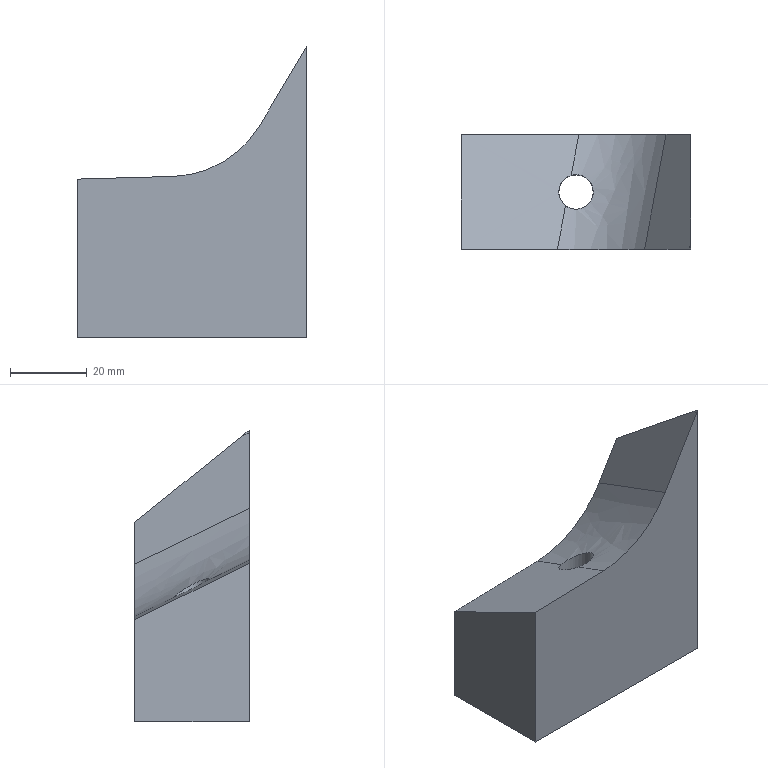Part | NX | features solid 2 | 1 solid | 10 faces | box 60.003 x 30 x 76.186 mm | volume 68995 mm3 | plane 5 | spline 4 | cylinder 1 | commonest cylinder face diameters 9 x1
STEP:
#1=CARTESIAN_POINT('',(-584.5,125.,-55.));
#2=VERTEX_POINT('',#1);
#3=CARTESIAN_POINT('',(-580.,125.,-55.));
#4=DIRECTION('',(0.,0.,-1.));
#5=DIRECTION('',(-1.,0.,0.));
#6=AXIS2_PLACEMENT_3D('',#3,#4,#5);
#7=CIRCLE('',#6,4.5);
#8=EDGE_CURVE('',#2,#2,#7,.T.);
#9=ORIENTED_EDGE('',*,*,#8,.F.);
#10=EDGE_LOOP('',(#9));
#11=FACE_BOUND('',#10,.T.);
#12=CARTESIAN_POINT('',(-610.,140.,-55.));
#13=VERTEX_POINT('',#12);
#14=CARTESIAN_POINT('',(-550.,140.,-55.));
#15=VERTEX_POINT('',#14);
#16=CARTESIAN_POINT('',(-615.,140.,-55.));
#17=DIRECTION('',(1.,0.,0.));
#18=VECTOR('',#17,1000.);
#19=LINE('',#16,#18);
#20=EDGE_CURVE('',#13,#15,#19,.T.);
#21=ORIENTED_EDGE('',*,*,#20,.T.);
#22=CARTESIAN_POINT('',(-550.,110.,-55.));
#23=VERTEX_POINT('',#22);
#24=CARTESIAN_POINT('',(-550.,140.,-55.));
#25=DIRECTION('',(0.,-1.,0.));
#26=VECTOR('',#25,1000.);
#27=LINE('',#24,#26);
#28=EDGE_CURVE('',#15,#23,#27,.T.);
#29=ORIENTED_EDGE('',*,*,#28,.T.);
#30=CARTESIAN_POINT('',(-610.,110.,-55.));
#31=VERTEX_POINT('',#30);
#32=CARTESIAN_POINT('',(-540.,110.,-55.));
#33=DIRECTION('',(-1.,0.,0.));
#34=VECTOR('',#33,1000.);
#35=LINE('',#32,#34);
#36=EDGE_CURVE('',#23,#31,#35,.T.);
#37=ORIENTED_EDGE('',*,*,#36,.T.);
#38=CARTESIAN_POINT('',(-610.,110.,-55.));
#39=DIRECTION('',(0.,1.,0.));
#40=VECTOR('',#39,1000.);
#41=LINE('',#38,#40);
#42=EDGE_CURVE('',#31,#13,#41,.T.);
#43=ORIENTED_EDGE('',*,*,#42,.T.);
#44=EDGE_LOOP('',(#21,#29,#37,#43));
#45=FACE_BOUND('',#44,.T.);
#46=CARTESIAN_POINT('',(-540.,140.,-55.));
#47=DIRECTION('',(0.,0.,-1.));
#48=DIRECTION('',(-1.,0.,0.));
#49=AXIS2_PLACEMENT_3D('',#46,#47,#48);
#50=PLANE('',#49);
#51=ADVANCED_FACE('',(#11,#45),#50,.T.);
#52=CARTESIAN_POINT('',(-610.,110.,-13.535));
#53=VERTEX_POINT('',#52);
#54=CARTESIAN_POINT('',(-610.,110.,-50.));
#55=DIRECTION('',(0.,0.,1.));
#56=VECTOR('',#55,1000.);
#57=LINE('',#54,#56);
#58=EDGE_CURVE('',#31,#53,#57,.T.);
#59=ORIENTED_EDGE('',*,*,#58,.T.);
#60=CARTESIAN_POINT('',(-610.,140.,-28.38));
#61=VERTEX_POINT('',#60);
#62=CARTESIAN_POINT('',(-610.,124.496,-20.708));
#63=DIRECTION('',(0.,-0.8963,0.4435));
#64=VECTOR('',#63,1000.);
#65=LINE('',#62,#64);
#66=EDGE_CURVE('',#53,#61,#65,.F.);
#67=ORIENTED_EDGE('',*,*,#66,.T.);
#68=CARTESIAN_POINT('',(-610.,140.,-50.));
#69=DIRECTION('',(0.,0.,1.));
#70=VECTOR('',#69,1000.);
#71=LINE('',#68,#70);
#72=EDGE_CURVE('',#13,#61,#71,.T.);
#73=ORIENTED_EDGE('',*,*,#72,.F.);
#74=ORIENTED_EDGE('',*,*,#42,.F.);
#75=EDGE_LOOP('',(#59,#67,#73,#74));
#76=FACE_BOUND('',#75,.T.);
#77=CARTESIAN_POINT('',(-610.,110.,-50.));
#78=DIRECTION('',(1.,0.,0.));
#79=DIRECTION('',(0.,0.,-1.));
#80=AXIS2_PLACEMENT_3D('',#77,#78,#79);
#81=PLANE('',#80);
#82=ADVANCED_FACE('',(#76),#81,.F.);
#83=CARTESIAN_POINT('',(-562.096,110.,0.8233));
#84=VERTEX_POINT('',#83);
#85=CARTESIAN_POINT('',(-584.853,110.,-12.829));
#86=VERTEX_POINT('',#85);
#87=CARTESIAN_POINT('',(-562.096,110.,0.8233));
#88=CARTESIAN_POINT('',(-564.471,110.,-3.178));
#89=CARTESIAN_POINT('',(-569.402,110.,-8.281));
#90=CARTESIAN_POINT('',(-577.942,110.,-12.047));
#91=CARTESIAN_POINT('',(-582.526,110.,-12.763));
#92=CARTESIAN_POINT('',(-584.853,110.,-12.829));
#93=B_SPLINE_CURVE_WITH_KNOTS('',3,(#87,#88,#89,#90,#91,#92),.UNSPECIFIED.,.F.,.F.,(4,1,1,4),(0.,0.01386,0.02078,0.02771),.UNSPECIFIED.);
#94=EDGE_CURVE('',#84,#86,#93,.T.);
#95=ORIENTED_EDGE('',*,*,#94,.T.);
#96=CARTESIAN_POINT('',(-541.078,110.,-11.6));
#97=DIRECTION('',(0.9996,0.,0.02806));
#98=VECTOR('',#97,1000.);
#99=LINE('',#96,#98);
#100=EDGE_CURVE('',#86,#53,#99,.F.);
#101=ORIENTED_EDGE('',*,*,#100,.T.);
#102=ORIENTED_EDGE('',*,*,#58,.F.);
#103=ORIENTED_EDGE('',*,*,#36,.F.);
#104=CARTESIAN_POINT('',(-550.,110.,21.186));
#105=VERTEX_POINT('',#104);
#106=CARTESIAN_POINT('',(-550.,110.,-50.));
#107=DIRECTION('',(0.,0.,1.));
#108=VECTOR('',#107,1000.);
#109=LINE('',#106,#108);
#110=EDGE_CURVE('',#23,#105,#109,.T.);
#111=ORIENTED_EDGE('',*,*,#110,.T.);
#112=CARTESIAN_POINT('',(-550.378,110.,20.569));
#113=VERTEX_POINT('',#112);
#114=CARTESIAN_POINT('',(-550.,110.,21.186));
#115=CARTESIAN_POINT('',(-550.129,110.,20.981));
#116=CARTESIAN_POINT('',(-550.256,110.,20.773));
#117=CARTESIAN_POINT('',(-550.38,110.,20.564));
#118=B_SPLINE_CURVE_WITH_KNOTS('',3,(#114,#115,#116,#117),.UNSPECIFIED.,.F.,.F.,(4,4),(0.,0.0007289),.UNSPECIFIED.);
#119=EDGE_CURVE('',#105,#113,#118,.T.);
#120=ORIENTED_EDGE('',*,*,#119,.T.);
#121=CARTESIAN_POINT('',(-578.647,110.,-27.064));
#122=DIRECTION('',(0.5104,0.,0.86));
#123=VECTOR('',#122,1000.);
#124=LINE('',#121,#123);
#125=EDGE_CURVE('',#113,#84,#124,.F.);
#126=ORIENTED_EDGE('',*,*,#125,.T.);
#127=EDGE_LOOP('',(#95,#101,#102,#103,#111,#120,#126));
#128=FACE_BOUND('',#127,.T.);
#129=CARTESIAN_POINT('',(-540.,110.,-50.));
#130=DIRECTION('',(0.,1.,0.));
#131=DIRECTION('',(0.,0.,1.));
#132=AXIS2_PLACEMENT_3D('',#129,#130,#131);
#133=PLANE('',#132);
#134=ADVANCED_FACE('',(#128),#133,.F.);
#135=CARTESIAN_POINT('',(-550.,140.,-2.908));
#136=VERTEX_POINT('',#135);
#137=CARTESIAN_POINT('',(-550.,140.,-50.));
#138=DIRECTION('',(0.,0.,1.));
#139=VECTOR('',#138,1000.);
#140=LINE('',#137,#139);
#141=EDGE_CURVE('',#15,#136,#140,.T.);
#142=ORIENTED_EDGE('',*,*,#141,.T.);
#143=CARTESIAN_POINT('',(-550.,111.813,19.748));
#144=VERTEX_POINT('',#143);
#145=CARTESIAN_POINT('',(-550.,162.995,-21.39));
#146=DIRECTION('',(0.,0.7794,-0.6265));
#147=VECTOR('',#146,1000.);
#148=LINE('',#145,#147);
#149=EDGE_CURVE('',#136,#144,#148,.F.);
#150=ORIENTED_EDGE('',*,*,#149,.T.);
#151=CARTESIAN_POINT('',(-550.,111.819,19.743));
#152=CARTESIAN_POINT('',(-550.,111.216,20.228));
#153=CARTESIAN_POINT('',(-550.,110.609,20.709));
#154=CARTESIAN_POINT('',(-550.,110.,21.186));
#155=B_SPLINE_CURVE_WITH_KNOTS('',3,(#151,#152,#153,#154),.UNSPECIFIED.,.F.,.F.,(4,4),(0.,0.002322),.UNSPECIFIED.);
#156=EDGE_CURVE('',#144,#105,#155,.T.);
#157=ORIENTED_EDGE('',*,*,#156,.T.);
#158=ORIENTED_EDGE('',*,*,#110,.F.);
#159=ORIENTED_EDGE('',*,*,#28,.F.);
#160=EDGE_LOOP('',(#142,#150,#157,#158,#159));
#161=FACE_BOUND('',#160,.T.);
#162=CARTESIAN_POINT('',(-550.,140.,-50.));
#163=DIRECTION('',(-1.,0.,0.));
#164=DIRECTION('',(0.,0.,1.));
#165=AXIS2_PLACEMENT_3D('',#162,#163,#164);
#166=PLANE('',#165);
#167=ADVANCED_FACE('',(#161),#166,.F.);
#168=CARTESIAN_POINT('',(-579.26,140.,-27.518));
#169=VERTEX_POINT('',#168);
#170=CARTESIAN_POINT('',(-556.503,140.,-13.866));
#171=VERTEX_POINT('',#170);
#172=CARTESIAN_POINT('',(-579.26,140.,-27.518));
#173=CARTESIAN_POINT('',(-574.607,140.,-27.387));
#174=CARTESIAN_POINT('',(-565.491,140.,-24.701));
#175=CARTESIAN_POINT('',(-558.877,140.,-17.866));
#176=CARTESIAN_POINT('',(-556.503,140.,-13.866));
#177=B_SPLINE_CURVE_WITH_KNOTS('',3,(#172,#173,#174,#175,#176),.UNSPECIFIED.,.F.,.F.,(4,1,4),(0.,0.01384,0.02768),.UNSPECIFIED.);
#178=EDGE_CURVE('',#169,#171,#177,.T.);
#179=ORIENTED_EDGE('',*,*,#178,.T.);
#180=CARTESIAN_POINT('',(-587.6,140.,-66.262));
#181=DIRECTION('',(-0.5104,0.,-0.86));
#182=VECTOR('',#181,1000.);
#183=LINE('',#180,#182);
#184=EDGE_CURVE('',#171,#136,#183,.F.);
#185=ORIENTED_EDGE('',*,*,#184,.T.);
#186=ORIENTED_EDGE('',*,*,#141,.F.);
#187=ORIENTED_EDGE('',*,*,#20,.F.);
#188=ORIENTED_EDGE('',*,*,#72,.T.);
#189=CARTESIAN_POINT('',(-615.602,140.,-28.538));
#190=DIRECTION('',(-0.9996,0.,-0.02806));
#191=VECTOR('',#190,1000.);
#192=LINE('',#189,#191);
#193=EDGE_CURVE('',#61,#169,#192,.F.);
#194=ORIENTED_EDGE('',*,*,#193,.T.);
#195=EDGE_LOOP('',(#179,#185,#186,#187,#188,#194));
#196=FACE_BOUND('',#195,.T.);
#197=CARTESIAN_POINT('',(-615.,140.,-50.));
#198=DIRECTION('',(0.,-1.,0.));
#199=DIRECTION('',(0.,0.,-1.));
#200=AXIS2_PLACEMENT_3D('',#197,#198,#199);
#201=PLANE('',#200);
#202=ADVANCED_FACE('',(#196),#201,.F.);
#203=ORIENTED_EDGE('',*,*,#184,.F.);
#204=CARTESIAN_POINT('',(-556.503,140.,-13.866));
#205=CARTESIAN_POINT('',(-558.368,130.,-8.969));
#206=CARTESIAN_POINT('',(-560.232,120.,-4.073));
#207=CARTESIAN_POINT('',(-562.096,110.,0.8233));
#208=B_SPLINE_CURVE_WITH_KNOTS('',3,(#204,#205,#206,#207),.UNSPECIFIED.,.F.,.F.,(4,4),(0.1493,0.4089),.UNSPECIFIED.);
#209=EDGE_CURVE('',#171,#84,#208,.T.);
#210=ORIENTED_EDGE('',*,*,#209,.T.);
#211=ORIENTED_EDGE('',*,*,#125,.F.);
#212=CARTESIAN_POINT('',(-550.375,110.001,20.572));
#213=CARTESIAN_POINT('',(-550.251,110.602,20.297));
#214=CARTESIAN_POINT('',(-550.125,111.204,20.026));
#215=CARTESIAN_POINT('',(-549.997,111.807,19.757));
#216=B_SPLINE_CURVE_WITH_KNOTS('',3,(#212,#213,#214,#215),.UNSPECIFIED.,.F.,.F.,(4,4),(0.3383,0.3557),.UNSPECIFIED.);
#217=EDGE_CURVE('',#113,#144,#216,.T.);
#218=ORIENTED_EDGE('',*,*,#217,.T.);
#219=ORIENTED_EDGE('',*,*,#149,.F.);
#220=EDGE_LOOP('',(#203,#210,#211,#218,#219));
#221=FACE_BOUND('',#220,.T.);
#222=CARTESIAN_POINT('',(-554.754,102.228,19.441));
#223=CARTESIAN_POINT('',(-569.709,117.54,-18.064));
#224=CARTESIAN_POINT('',(-539.117,129.112,24.181));
#225=CARTESIAN_POINT('',(-554.072,144.423,-13.324));
#226=B_SPLINE_SURFACE_WITH_KNOTS('',1,1,((#222,#223),(#224,#225)),.PLANE_SURF.,.F.,.F.,.F.,(2,2),(2,2),(0.4546,0.6841),(0.4055,0.8654),.PIECEWISE_BEZIER_KNOTS.);
#227=ADVANCED_FACE('',(#221),#226,.T.);
#228=CARTESIAN_POINT('',(-581.251,129.323,-22.29));
#229=VERTEX_POINT('',#228);
#230=CARTESIAN_POINT('',(-579.26,140.,-27.518));
#231=CARTESIAN_POINT('',(-579.924,136.441,-25.775));
#232=CARTESIAN_POINT('',(-580.587,132.882,-24.032));
#233=CARTESIAN_POINT('',(-581.251,129.323,-22.29));
#234=B_SPLINE_CURVE_WITH_KNOTS('',3,(#230,#231,#232,#233),.UNSPECIFIED.,.F.,.F.,(4,4),(0.1327,0.2251),.UNSPECIFIED.);
#235=EDGE_CURVE('',#229,#169,#234,.F.);
#236=ORIENTED_EDGE('',*,*,#235,.F.);
#237=CARTESIAN_POINT('',(-582.724,121.418,-18.419));
#238=VERTEX_POINT('',#237);
#239=CARTESIAN_POINT('',(-581.251,129.323,-22.29));
#240=CARTESIAN_POINT('',(-580.47,129.549,-22.38));
#241=CARTESIAN_POINT('',(-578.782,129.553,-22.265));
#242=CARTESIAN_POINT('',(-576.762,128.373,-21.312));
#243=CARTESIAN_POINT('',(-575.612,126.566,-20.063));
#244=CARTESIAN_POINT('',(-575.361,124.437,-18.832));
#245=CARTESIAN_POINT('',(-576.162,122.273,-17.892));
#246=CARTESIAN_POINT('',(-578.1,120.669,-17.527));
#247=CARTESIAN_POINT('',(-580.602,120.32,-17.758));
#248=CARTESIAN_POINT('',(-582.104,120.947,-18.169));
#249=CARTESIAN_POINT('',(-582.724,121.418,-18.419));
#250=B_SPLINE_CURVE_WITH_KNOTS('',3,(#239,#240,#241,#242,#243,#244,#245,#246,#247,#248,#249),.UNSPECIFIED.,.F.,.F.,(4,1,1,1,1,1,1,1,4),(0.,0.002419,0.004838,0.007256,0.009675,0.01209,0.01451,0.01693,0.01935),.UNSPECIFIED.);
#251=EDGE_CURVE('',#229,#238,#250,.T.);
#252=ORIENTED_EDGE('',*,*,#251,.T.);
#253=CARTESIAN_POINT('',(-582.724,121.418,-18.419));
#254=CARTESIAN_POINT('',(-583.434,117.612,-16.556));
#255=CARTESIAN_POINT('',(-584.143,113.806,-14.692));
#256=CARTESIAN_POINT('',(-584.853,110.,-12.829));
#257=B_SPLINE_CURVE_WITH_KNOTS('',3,(#253,#254,#255,#256),.UNSPECIFIED.,.F.,.F.,(4,4),(0.2935,0.3924),.UNSPECIFIED.);
#258=EDGE_CURVE('',#86,#238,#257,.F.);
#259=ORIENTED_EDGE('',*,*,#258,.F.);
#260=ORIENTED_EDGE('',*,*,#94,.F.);
#261=ORIENTED_EDGE('',*,*,#209,.F.);
#262=ORIENTED_EDGE('',*,*,#178,.F.);
#263=EDGE_LOOP('',(#236,#252,#259,#260,#261,#262));
#264=FACE_BOUND('',#263,.T.);
#265=CARTESIAN_POINT('',(-579.097,140.875,-27.946));
#266=CARTESIAN_POINT('',(-585.247,107.888,-11.795));
#267=CARTESIAN_POINT('',(-569.767,139.578,-27.042));
#268=CARTESIAN_POINT('',(-575.917,106.592,-10.891));
#269=CARTESIAN_POINT('',(-561.498,140.264,-22.494));
#270=CARTESIAN_POINT('',(-567.648,107.277,-6.343));
#271=CARTESIAN_POINT('',(-555.983,142.791,-15.232));
#272=CARTESIAN_POINT('',(-562.133,109.804,0.919));
#273=(BOUNDED_SURFACE()B_SPLINE_SURFACE(3,1,((#265,#266),(#267,#268),(#269,#270),(#271,#272)),.CYLINDRICAL_SURF.,.F.,.F.,.F.)B_SPLINE_SURFACE_WITH_KNOTS((4,4),(2,2),(0.,1.),(0.1252,0.4106),.PIECEWISE_BEZIER_KNOTS.)GEOMETRIC_REPRESENTATION_ITEM()RATIONAL_B_SPLINE_SURFACE(((1.,1.),(0.9317,0.9317),(0.9317,0.9317),(1.,1.)))REPRESENTATION_ITEM('')SURFACE());
#274=ADVANCED_FACE('',(#264),#273,.F.);
#275=ORIENTED_EDGE('',*,*,#156,.F.);
#276=ORIENTED_EDGE('',*,*,#217,.F.);
#277=ORIENTED_EDGE('',*,*,#119,.F.);
#278=EDGE_LOOP('',(#275,#276,#277));
#279=FACE_BOUND('',#278,.T.);
#280=CARTESIAN_POINT('',(-549.582,111.981,20.298));
#281=CARTESIAN_POINT('',(-549.667,111.952,20.187));
#282=CARTESIAN_POINT('',(-549.75,111.922,20.075));
#283=CARTESIAN_POINT('',(-549.833,111.892,19.963));
#284=CARTESIAN_POINT('',(-549.916,111.861,19.85));
#285=CARTESIAN_POINT('',(-549.997,111.831,19.738));
#286=CARTESIAN_POINT('',(-549.667,111.582,20.475));
#287=CARTESIAN_POINT('',(-549.752,111.552,20.364));
#288=CARTESIAN_POINT('',(-549.836,111.522,20.253));
#289=CARTESIAN_POINT('',(-549.919,111.492,20.141));
#290=CARTESIAN_POINT('',(-550.001,111.461,20.029));
#291=CARTESIAN_POINT('',(-550.083,111.43,19.916));
#292=CARTESIAN_POINT('',(-549.752,111.183,20.653));
#293=CARTESIAN_POINT('',(-549.836,111.153,20.543));
#294=CARTESIAN_POINT('',(-549.92,111.123,20.432));
#295=CARTESIAN_POINT('',(-550.003,111.092,20.32));
#296=CARTESIAN_POINT('',(-550.085,111.061,20.208));
#297=CARTESIAN_POINT('',(-550.167,111.03,20.096));
#298=CARTESIAN_POINT('',(-549.835,110.784,20.833));
#299=CARTESIAN_POINT('',(-549.92,110.754,20.722));
#300=CARTESIAN_POINT('',(-550.004,110.724,20.612));
#301=CARTESIAN_POINT('',(-550.087,110.693,20.5));
#302=CARTESIAN_POINT('',(-550.169,110.661,20.389));
#303=CARTESIAN_POINT('',(-550.251,110.63,20.277));
#304=CARTESIAN_POINT('',(-549.918,110.387,21.013));
#305=CARTESIAN_POINT('',(-550.003,110.356,20.903));
#306=CARTESIAN_POINT('',(-550.086,110.325,20.793));
#307=CARTESIAN_POINT('',(-550.169,110.294,20.682));
#308=CARTESIAN_POINT('',(-550.251,110.262,20.57));
#309=CARTESIAN_POINT('',(-550.333,110.23,20.458));
#310=CARTESIAN_POINT('',(-550.,109.989,21.195));
#311=CARTESIAN_POINT('',(-550.084,109.958,21.085));
#312=CARTESIAN_POINT('',(-550.168,109.927,20.975));
#313=CARTESIAN_POINT('',(-550.251,109.896,20.864));
#314=CARTESIAN_POINT('',(-550.333,109.864,20.753));
#315=CARTESIAN_POINT('',(-550.415,109.832,20.642));
#316=B_SPLINE_SURFACE_WITH_KNOTS('',5,5,((#280,#281,#282,#283,#284,#285),(#286,#287,#288,#289,#290,#291),(#292,#293,#294,#295,#296,#297),(#298,#299,#300,#301,#302,#303),(#304,#305,#306,#307,#308,#309),(#310,#311,#312,#313,#314,#315)),.UNSPECIFIED.,.F.,.F.,.F.,(6,6),(6,6),(0.6436,0.6629),(0.9469,1.),.PIECEWISE_BEZIER_KNOTS.);
#317=ADVANCED_FACE('',(#279),#316,.F.);
#318=ORIENTED_EDGE('',*,*,#258,.T.);
#319=CARTESIAN_POINT('',(-582.724,121.418,-18.419));
#320=CARTESIAN_POINT('',(-584.082,122.451,-18.968));
#321=CARTESIAN_POINT('',(-585.351,125.852,-20.687));
#322=CARTESIAN_POINT('',(-582.969,128.826,-22.092));
#323=CARTESIAN_POINT('',(-581.251,129.323,-22.29));
#324=B_SPLINE_CURVE_WITH_KNOTS('',3,(#319,#320,#321,#322,#323),.UNSPECIFIED.,.F.,.F.,(4,1,4),(0.003896,0.009237,0.01458),.UNSPECIFIED.);
#325=EDGE_CURVE('',#238,#229,#324,.T.);
#326=ORIENTED_EDGE('',*,*,#325,.T.);
#327=ORIENTED_EDGE('',*,*,#235,.T.);
#328=ORIENTED_EDGE('',*,*,#193,.F.);
#329=ORIENTED_EDGE('',*,*,#66,.F.);
#330=ORIENTED_EDGE('',*,*,#100,.F.);
#331=EDGE_LOOP('',(#318,#326,#327,#328,#329,#330));
#332=FACE_BOUND('',#331,.T.);
#333=CARTESIAN_POINT('',(-610.,140.182,-28.47));
#334=CARTESIAN_POINT('',(-579.076,140.527,-27.773));
#335=CARTESIAN_POINT('',(-610.,109.538,-13.306));
#336=CARTESIAN_POINT('',(-579.076,109.883,-12.608));
#337=B_SPLINE_SURFACE_WITH_KNOTS('',1,1,((#333,#334),(#335,#336)),.PLANE_SURF.,.F.,.F.,.F.,(2,2),(2,2),(0.2725,0.4269),(0.5436,0.955),.PIECEWISE_BEZIER_KNOTS.);
#338=ADVANCED_FACE('',(#332),#337,.T.);
#339=ORIENTED_EDGE('',*,*,#8,.T.);
#340=EDGE_LOOP('',(#339));
#341=FACE_BOUND('',#340,.T.);
#342=ORIENTED_EDGE('',*,*,#325,.F.);
#343=ORIENTED_EDGE('',*,*,#251,.F.);
#344=EDGE_LOOP('',(#342,#343));
#345=FACE_BOUND('',#344,.T.);
#346=CARTESIAN_POINT('',(-580.,125.,-65.));
#347=DIRECTION('',(0.,0.,1.));
#348=DIRECTION('',(-1.,0.,0.));
#349=AXIS2_PLACEMENT_3D('',#346,#347,#348);
#350=CYLINDRICAL_SURFACE('',#349,4.5);
#351=ADVANCED_FACE('',(#341,#345),#350,.F.);
#352=CLOSED_SHELL('',(#51,#82,#134,#167,#202,#227,#274,#317,#338,#351));
#353=MANIFOLD_SOLID_BREP('',#352);
#354=(LENGTH_UNIT()NAMED_UNIT(*)SI_UNIT(.MILLI.,.METRE.));
#355=UNCERTAINTY_MEASURE_WITH_UNIT(LENGTH_MEASURE(0.1083),#354,'','');
#356=(NAMED_UNIT(*)PLANE_ANGLE_UNIT()SI_UNIT($,.RADIAN.));
#357=(NAMED_UNIT(*)SI_UNIT($,.STERADIAN.)SOLID_ANGLE_UNIT());
#358=(GEOMETRIC_REPRESENTATION_CONTEXT(3)GLOBAL_UNCERTAINTY_ASSIGNED_CONTEXT((#355))GLOBAL_UNIT_ASSIGNED_CONTEXT((#354,#356,#357))REPRESENTATION_CONTEXT('',''));
#359=ADVANCED_BREP_SHAPE_REPRESENTATION('',(#353),#358);